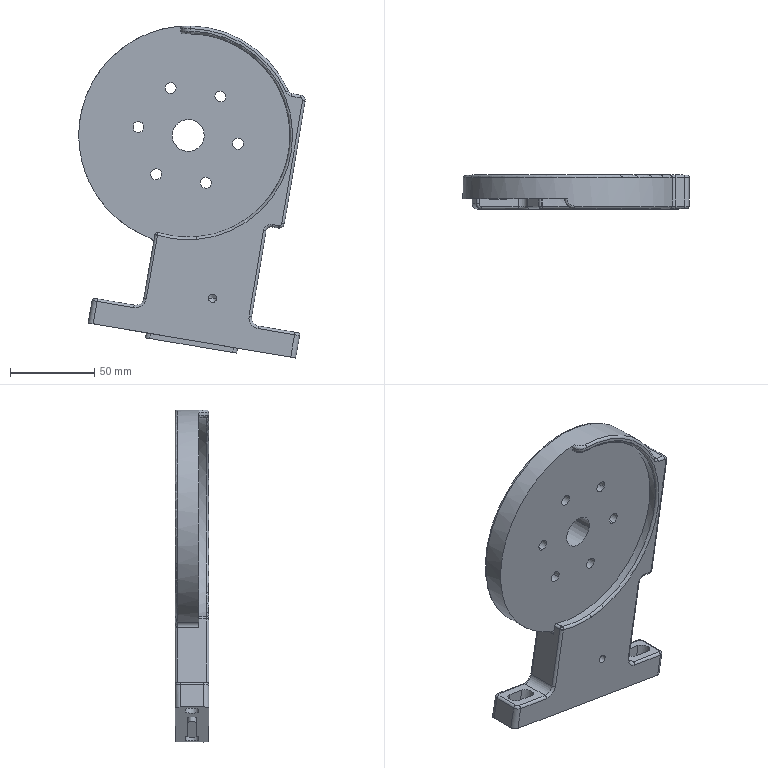Part | SolidWorks | features BaseBody 1 | 1 solid | 130 faces | box 134.403 x 20 x 197.23 mm | volume 283625 mm3 | cylinder 70 | plane 26 | torus 24 | cone 6 | spline 3 | sphere 1 | commonest cylinder face diameters 3 x18 6.5 x12 11 x12 6 x9 5 x4 5.2 x4